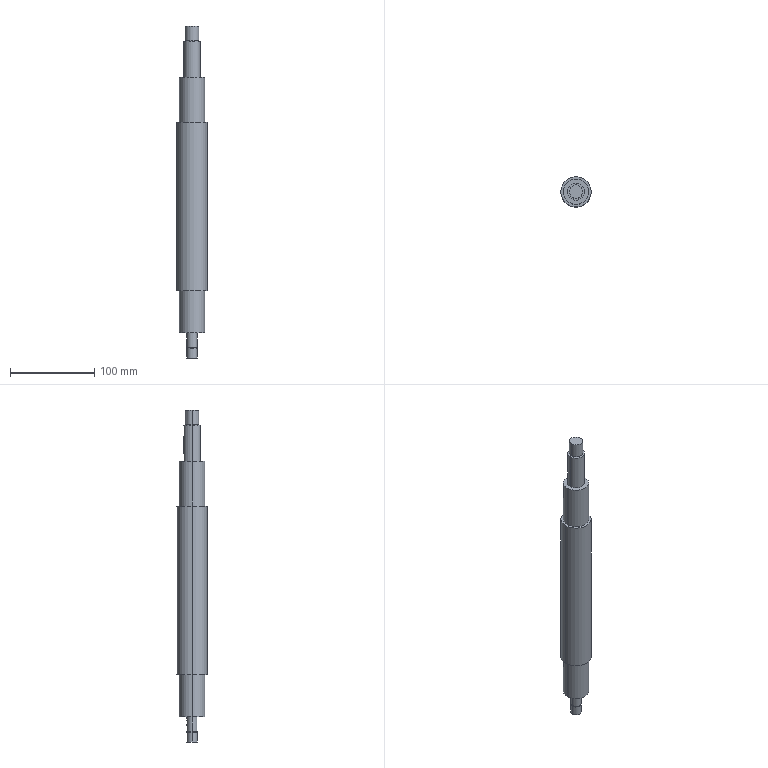Part | SolidWorks | features ICE 9, Extrusion 1 | 1 solid | 40 faces | box 36 x 36 x 394 mm | volume 296771 mm3 | cylinder 24 | plane 16 | commonest cylinder face diameters 2 x6 12 x4 30 x4 10 x2 14 x2 16 x2
STEP:
#1=CARTESIAN_POINT('',(8.,0.,364.));
#2=VERTEX_POINT('',#1);
#3=CARTESIAN_POINT('',(-8.,0.,364.));
#4=VERTEX_POINT('',#3);
#5=CARTESIAN_POINT('',(0.,0.,364.));
#6=DIRECTION('',(0.,0.,1.));
#7=DIRECTION('',(1.,0.,0.));
#8=AXIS2_PLACEMENT_3D('',#5,#6,#7);
#9=CIRCLE('',#8,8.);
#10=EDGE_CURVE('',#2,#4,#9,.T.);
#11=ORIENTED_EDGE('',*,*,#10,.F.);
#12=CARTESIAN_POINT('',(8.,0.,347.));
#13=VERTEX_POINT('',#12);
#14=CARTESIAN_POINT('',(8.,0.,364.));
#15=DIRECTION('',(0.,0.,-1.));
#16=VECTOR('',#15,1000.);
#17=LINE('',#14,#16);
#18=EDGE_CURVE('',#2,#13,#17,.T.);
#19=ORIENTED_EDGE('',*,*,#18,.T.);
#20=CARTESIAN_POINT('',(-8.,0.,347.));
#21=VERTEX_POINT('',#20);
#22=CARTESIAN_POINT('',(0.,0.,347.));
#23=DIRECTION('',(0.,0.,1.));
#24=DIRECTION('',(1.,0.,0.));
#25=AXIS2_PLACEMENT_3D('',#22,#23,#24);
#26=CIRCLE('',#25,8.);
#27=EDGE_CURVE('',#13,#21,#26,.T.);
#28=ORIENTED_EDGE('',*,*,#27,.T.);
#29=CARTESIAN_POINT('',(-8.,0.,364.));
#30=DIRECTION('',(0.,0.,-1.));
#31=VECTOR('',#30,1000.);
#32=LINE('',#29,#31);
#33=EDGE_CURVE('',#4,#21,#32,.T.);
#34=ORIENTED_EDGE('',*,*,#33,.F.);
#35=EDGE_LOOP('',(#11,#19,#28,#34));
#36=FACE_OUTER_BOUND('',#35,.T.);
#37=CARTESIAN_POINT('',(0.,0.,364.));
#38=DIRECTION('',(0.,0.,-1.));
#39=DIRECTION('',(-1.,0.,0.));
#40=AXIS2_PLACEMENT_3D('',#37,#38,#39);
#41=CYLINDRICAL_SURFACE('',#40,8.);
#42=ADVANCED_FACE('',(#36),#41,.T.);
#43=CARTESIAN_POINT('',(7.,0.,347.));
#44=VERTEX_POINT('',#43);
#45=CARTESIAN_POINT('',(-7.,0.,347.));
#46=VERTEX_POINT('',#45);
#47=CARTESIAN_POINT('',(0.,0.,347.));
#48=DIRECTION('',(0.,0.,1.));
#49=DIRECTION('',(1.,0.,0.));
#50=AXIS2_PLACEMENT_3D('',#47,#48,#49);
#51=CIRCLE('',#50,7.);
#52=EDGE_CURVE('',#44,#46,#51,.T.);
#53=ORIENTED_EDGE('',*,*,#52,.F.);
#54=CARTESIAN_POINT('',(7.,0.,346.));
#55=VERTEX_POINT('',#54);
#56=CARTESIAN_POINT('',(7.,0.,347.));
#57=DIRECTION('',(0.,0.,-1.));
#58=VECTOR('',#57,1000.);
#59=LINE('',#56,#58);
#60=EDGE_CURVE('',#44,#55,#59,.T.);
#61=ORIENTED_EDGE('',*,*,#60,.T.);
#62=CARTESIAN_POINT('',(-7.,0.,346.));
#63=VERTEX_POINT('',#62);
#64=CARTESIAN_POINT('',(0.,0.,346.));
#65=DIRECTION('',(0.,0.,1.));
#66=DIRECTION('',(1.,0.,0.));
#67=AXIS2_PLACEMENT_3D('',#64,#65,#66);
#68=CIRCLE('',#67,7.);
#69=EDGE_CURVE('',#55,#63,#68,.T.);
#70=ORIENTED_EDGE('',*,*,#69,.T.);
#71=CARTESIAN_POINT('',(-7.,0.,347.));
#72=DIRECTION('',(0.,0.,-1.));
#73=VECTOR('',#72,1000.);
#74=LINE('',#71,#73);
#75=EDGE_CURVE('',#46,#63,#74,.T.);
#76=ORIENTED_EDGE('',*,*,#75,.F.);
#77=EDGE_LOOP('',(#53,#61,#70,#76));
#78=FACE_OUTER_BOUND('',#77,.T.);
#79=CARTESIAN_POINT('',(0.,0.,347.));
#80=DIRECTION('',(0.,0.,-1.));
#81=DIRECTION('',(-1.,0.,0.));
#82=AXIS2_PLACEMENT_3D('',#79,#80,#81);
#83=CYLINDRICAL_SURFACE('',#82,7.);
#84=ADVANCED_FACE('',(#78),#83,.T.);
#85=CARTESIAN_POINT('',(1.,9.95,313.));
#86=VERTEX_POINT('',#85);
#87=CARTESIAN_POINT('',(0.,10.,312.));
#88=VERTEX_POINT('',#87);
#89=CARTESIAN_POINT('',(1.,9.95,313.));
#90=CARTESIAN_POINT('',(1.,9.95,312.868));
#91=CARTESIAN_POINT('',(0.9739,9.953,312.738));
#92=CARTESIAN_POINT('',(0.8734,9.962,312.496));
#93=CARTESIAN_POINT('',(0.7991,9.968,312.385));
#94=CARTESIAN_POINT('',(0.6146,9.982,312.2));
#95=CARTESIAN_POINT('',(0.503,9.988,312.126));
#96=CARTESIAN_POINT('',(0.2623,9.997,312.026));
#97=CARTESIAN_POINT('',(0.1306,10.,312.));
#98=CARTESIAN_POINT('',(0.,10.,312.));
#99=B_SPLINE_CURVE_WITH_KNOTS('',3,(#89,#90,#91,#92,#93,#94,#95,#96,#97,#98),.UNSPECIFIED.,.F.,.F.,(4,2,2,2,4),(0.,0.0003911,0.0007823,0.001173,0.001565),.UNSPECIFIED.);
#100=EDGE_CURVE('',#86,#88,#99,.T.);
#101=ORIENTED_EDGE('',*,*,#100,.T.);
#102=CARTESIAN_POINT('',(0.,9.,312.));
#103=VERTEX_POINT('',#102);
#104=CARTESIAN_POINT('',(0.,21.,312.));
#105=DIRECTION('',(0.,-1.,0.));
#106=VECTOR('',#105,1000.);
#107=LINE('',#104,#106);
#108=EDGE_CURVE('',#88,#103,#107,.T.);
#109=ORIENTED_EDGE('',*,*,#108,.T.);
#110=CARTESIAN_POINT('',(1.,9.,313.));
#111=VERTEX_POINT('',#110);
#112=CARTESIAN_POINT('',(0.,9.,313.));
#113=DIRECTION('',(0.,1.,0.));
#114=DIRECTION('',(0.,0.,1.));
#115=AXIS2_PLACEMENT_3D('',#112,#113,#114);
#116=CIRCLE('',#115,1.);
#117=EDGE_CURVE('',#111,#103,#116,.T.);
#118=ORIENTED_EDGE('',*,*,#117,.F.);
#119=CARTESIAN_POINT('',(1.,21.,313.));
#120=DIRECTION('',(0.,-1.,0.));
#121=VECTOR('',#120,1000.);
#122=LINE('',#119,#121);
#123=EDGE_CURVE('',#86,#111,#122,.T.);
#124=ORIENTED_EDGE('',*,*,#123,.F.);
#125=EDGE_LOOP('',(#101,#109,#118,#124));
#126=FACE_OUTER_BOUND('',#125,.T.);
#127=CARTESIAN_POINT('',(0.,21.,313.));
#128=DIRECTION('',(0.,-1.,0.));
#129=DIRECTION('',(0.,0.,-1.));
#130=AXIS2_PLACEMENT_3D('',#127,#128,#129);
#131=CYLINDRICAL_SURFACE('',#130,1.);
#132=ADVANCED_FACE('',(#126),#131,.F.);
#133=CARTESIAN_POINT('',(-6.,0.,-30.));
#134=VERTEX_POINT('',#133);
#135=CARTESIAN_POINT('',(6.,0.,-30.));
#136=VERTEX_POINT('',#135);
#137=CARTESIAN_POINT('',(0.,0.,-30.));
#138=DIRECTION('',(0.,0.,-1.));
#139=DIRECTION('',(-1.,0.,0.));
#140=AXIS2_PLACEMENT_3D('',#137,#138,#139);
#141=CIRCLE('',#140,6.);
#142=EDGE_CURVE('',#134,#136,#141,.T.);
#143=ORIENTED_EDGE('',*,*,#142,.F.);
#144=CARTESIAN_POINT('',(-6.,0.,-18.5));
#145=VERTEX_POINT('',#144);
#146=CARTESIAN_POINT('',(-6.,0.,-30.));
#147=DIRECTION('',(0.,0.,1.));
#148=VECTOR('',#147,1000.);
#149=LINE('',#146,#148);
#150=EDGE_CURVE('',#134,#145,#149,.T.);
#151=ORIENTED_EDGE('',*,*,#150,.T.);
#152=CARTESIAN_POINT('',(6.,0.,-18.5));
#153=VERTEX_POINT('',#152);
#154=CARTESIAN_POINT('',(0.,0.,-18.5));
#155=DIRECTION('',(0.,0.,-1.));
#156=DIRECTION('',(-1.,0.,0.));
#157=AXIS2_PLACEMENT_3D('',#154,#155,#156);
#158=CIRCLE('',#157,6.);
#159=EDGE_CURVE('',#145,#153,#158,.T.);
#160=ORIENTED_EDGE('',*,*,#159,.T.);
#161=CARTESIAN_POINT('',(6.,0.,-30.));
#162=DIRECTION('',(0.,0.,1.));
#163=VECTOR('',#162,1000.);
#164=LINE('',#161,#163);
#165=EDGE_CURVE('',#136,#153,#164,.T.);
#166=ORIENTED_EDGE('',*,*,#165,.F.);
#167=EDGE_LOOP('',(#143,#151,#160,#166));
#168=FACE_OUTER_BOUND('',#167,.T.);
#169=CARTESIAN_POINT('',(0.,0.,-30.));
#170=DIRECTION('',(0.,0.,1.));
#171=DIRECTION('',(1.,0.,0.));
#172=AXIS2_PLACEMENT_3D('',#169,#170,#171);
#173=CYLINDRICAL_SURFACE('',#172,6.);
#174=ADVANCED_FACE('',(#168),#173,.T.);
#175=CARTESIAN_POINT('',(-5.,0.,-17.5));
#176=VERTEX_POINT('',#175);
#177=CARTESIAN_POINT('',(5.,0.,-17.5));
#178=VERTEX_POINT('',#177);
#179=CARTESIAN_POINT('',(0.,0.,-17.5));
#180=DIRECTION('',(0.,0.,-1.));
#181=DIRECTION('',(-1.,0.,0.));
#182=AXIS2_PLACEMENT_3D('',#179,#180,#181);
#183=CIRCLE('',#182,5.);
#184=EDGE_CURVE('',#176,#178,#183,.T.);
#185=ORIENTED_EDGE('',*,*,#184,.T.);
#186=CARTESIAN_POINT('',(5.,0.,-18.5));
#187=VERTEX_POINT('',#186);
#188=CARTESIAN_POINT('',(5.,0.,-17.5));
#189=DIRECTION('',(0.,0.,-1.));
#190=VECTOR('',#189,1000.);
#191=LINE('',#188,#190);
#192=EDGE_CURVE('',#178,#187,#191,.T.);
#193=ORIENTED_EDGE('',*,*,#192,.T.);
#194=CARTESIAN_POINT('',(-5.,0.,-18.5));
#195=VERTEX_POINT('',#194);
#196=CARTESIAN_POINT('',(0.,0.,-18.5));
#197=DIRECTION('',(0.,0.,-1.));
#198=DIRECTION('',(-1.,0.,0.));
#199=AXIS2_PLACEMENT_3D('',#196,#197,#198);
#200=CIRCLE('',#199,5.);
#201=EDGE_CURVE('',#195,#187,#200,.T.);
#202=ORIENTED_EDGE('',*,*,#201,.F.);
#203=CARTESIAN_POINT('',(-5.,0.,-17.5));
#204=DIRECTION('',(0.,0.,-1.));
#205=VECTOR('',#204,1000.);
#206=LINE('',#203,#205);
#207=EDGE_CURVE('',#176,#195,#206,.T.);
#208=ORIENTED_EDGE('',*,*,#207,.F.);
#209=EDGE_LOOP('',(#185,#193,#202,#208));
#210=FACE_OUTER_BOUND('',#209,.T.);
#211=CARTESIAN_POINT('',(0.,0.,-17.5));
#212=DIRECTION('',(0.,0.,-1.));
#213=DIRECTION('',(-1.,0.,0.));
#214=AXIS2_PLACEMENT_3D('',#211,#212,#213);
#215=CYLINDRICAL_SURFACE('',#214,5.);
#216=ADVANCED_FACE('',(#210),#215,.T.);
#217=CARTESIAN_POINT('',(1.,5.916,-9.));
#218=VERTEX_POINT('',#217);
#219=CARTESIAN_POINT('',(0.,6.,-10.));
#220=VERTEX_POINT('',#219);
#221=CARTESIAN_POINT('',(1.,5.916,-9.));
#222=CARTESIAN_POINT('',(1.,5.916,-9.132));
#223=CARTESIAN_POINT('',(0.9738,5.921,-9.262));
#224=CARTESIAN_POINT('',(0.8733,5.936,-9.505));
#225=CARTESIAN_POINT('',(0.799,5.947,-9.615));
#226=CARTESIAN_POINT('',(0.6147,5.969,-9.799));
#227=CARTESIAN_POINT('',(0.5032,5.98,-9.874));
#228=CARTESIAN_POINT('',(0.2625,5.995,-9.974));
#229=CARTESIAN_POINT('',(0.1307,6.,-10.));
#230=CARTESIAN_POINT('',(0.,6.,-10.));
#231=B_SPLINE_CURVE_WITH_KNOTS('',3,(#221,#222,#223,#224,#225,#226,#227,#228,#229,#230),.UNSPECIFIED.,.F.,.F.,(4,2,2,2,4),(0.,0.0003916,0.0007832,0.001175,0.001566),.UNSPECIFIED.);
#232=EDGE_CURVE('',#218,#220,#231,.T.);
#233=ORIENTED_EDGE('',*,*,#232,.T.);
#234=CARTESIAN_POINT('',(0.,5.,-10.));
#235=VERTEX_POINT('',#234);
#236=CARTESIAN_POINT('',(0.,15.,-10.));
#237=DIRECTION('',(0.,-1.,0.));
#238=VECTOR('',#237,1000.);
#239=LINE('',#236,#238);
#240=EDGE_CURVE('',#220,#235,#239,.T.);
#241=ORIENTED_EDGE('',*,*,#240,.T.);
#242=CARTESIAN_POINT('',(1.,5.,-9.));
#243=VERTEX_POINT('',#242);
#244=CARTESIAN_POINT('',(0.,5.,-9.));
#245=DIRECTION('',(0.,1.,0.));
#246=DIRECTION('',(0.,0.,1.));
#247=AXIS2_PLACEMENT_3D('',#244,#245,#246);
#248=CIRCLE('',#247,1.);
#249=EDGE_CURVE('',#243,#235,#248,.T.);
#250=ORIENTED_EDGE('',*,*,#249,.F.);
#251=CARTESIAN_POINT('',(1.,15.,-9.));
#252=DIRECTION('',(0.,-1.,0.));
#253=VECTOR('',#252,1000.);
#254=LINE('',#251,#253);
#255=EDGE_CURVE('',#218,#243,#254,.T.);
#256=ORIENTED_EDGE('',*,*,#255,.F.);
#257=EDGE_LOOP('',(#233,#241,#250,#256));
#258=FACE_OUTER_BOUND('',#257,.T.);
#259=CARTESIAN_POINT('',(0.,15.,-9.));
#260=DIRECTION('',(0.,-1.,0.));
#261=DIRECTION('',(0.,0.,-1.));
#262=AXIS2_PLACEMENT_3D('',#259,#260,#261);
#263=CYLINDRICAL_SURFACE('',#262,1.);
#264=ADVANCED_FACE('',(#258),#263,.F.);
#265=CARTESIAN_POINT('',(15.,0.,303.));
#266=VERTEX_POINT('',#265);
#267=CARTESIAN_POINT('',(-15.,0.,303.));
#268=VERTEX_POINT('',#267);
#269=CARTESIAN_POINT('',(0.,0.,303.));
#270=DIRECTION('',(0.,0.,1.));
#271=DIRECTION('',(1.,0.,0.));
#272=AXIS2_PLACEMENT_3D('',#269,#270,#271);
#273=CIRCLE('',#272,15.);
#274=EDGE_CURVE('',#266,#268,#273,.T.);
#275=ORIENTED_EDGE('',*,*,#274,.F.);
#276=CARTESIAN_POINT('',(15.,0.,250.));
#277=VERTEX_POINT('',#276);
#278=CARTESIAN_POINT('',(15.,0.,303.));
#279=DIRECTION('',(0.,0.,-1.));
#280=VECTOR('',#279,1000.);
#281=LINE('',#278,#280);
#282=EDGE_CURVE('',#266,#277,#281,.T.);
#283=ORIENTED_EDGE('',*,*,#282,.T.);
#284=CARTESIAN_POINT('',(-15.,0.,250.));
#285=VERTEX_POINT('',#284);
#286=CARTESIAN_POINT('',(0.,0.,250.));
#287=DIRECTION('',(0.,0.,1.));
#288=DIRECTION('',(1.,0.,0.));
#289=AXIS2_PLACEMENT_3D('',#286,#287,#288);
#290=CIRCLE('',#289,15.);
#291=EDGE_CURVE('',#277,#285,#290,.T.);
#292=ORIENTED_EDGE('',*,*,#291,.T.);
#293=CARTESIAN_POINT('',(-15.,0.,303.));
#294=DIRECTION('',(0.,0.,-1.));
#295=VECTOR('',#294,1000.);
#296=LINE('',#293,#295);
#297=EDGE_CURVE('',#268,#285,#296,.T.);
#298=ORIENTED_EDGE('',*,*,#297,.F.);
#299=EDGE_LOOP('',(#275,#283,#292,#298));
#300=FACE_OUTER_BOUND('',#299,.T.);
#301=CARTESIAN_POINT('',(0.,0.,303.));
#302=DIRECTION('',(0.,0.,-1.));
#303=DIRECTION('',(-1.,0.,0.));
#304=AXIS2_PLACEMENT_3D('',#301,#302,#303);
#305=CYLINDRICAL_SURFACE('',#304,15.);
#306=ADVANCED_FACE('',(#300),#305,.T.);
#307=CARTESIAN_POINT('',(18.,0.,250.));
#308=VERTEX_POINT('',#307);
#309=CARTESIAN_POINT('',(-18.,0.,250.));
#310=VERTEX_POINT('',#309);
#311=CARTESIAN_POINT('',(0.,0.,250.));
#312=DIRECTION('',(0.,0.,1.));
#313=DIRECTION('',(1.,0.,0.));
#314=AXIS2_PLACEMENT_3D('',#311,#312,#313);
#315=CIRCLE('',#314,18.);
#316=EDGE_CURVE('',#308,#310,#315,.T.);
#317=ORIENTED_EDGE('',*,*,#316,.F.);
#318=CARTESIAN_POINT('',(18.,0.,50.));
#319=VERTEX_POINT('',#318);
#320=CARTESIAN_POINT('',(18.,0.,250.));
#321=DIRECTION('',(0.,0.,-1.));
#322=VECTOR('',#321,1000.);
#323=LINE('',#320,#322);
#324=EDGE_CURVE('',#308,#319,#323,.T.);
#325=ORIENTED_EDGE('',*,*,#324,.T.);
#326=CARTESIAN_POINT('',(-18.,0.,50.));
#327=VERTEX_POINT('',#326);
#328=CARTESIAN_POINT('',(0.,0.,50.));
#329=DIRECTION('',(0.,0.,1.));
#330=DIRECTION('',(1.,0.,0.));
#331=AXIS2_PLACEMENT_3D('',#328,#329,#330);
#332=CIRCLE('',#331,18.);
#333=EDGE_CURVE('',#319,#327,#332,.T.);
#334=ORIENTED_EDGE('',*,*,#333,.T.);
#335=CARTESIAN_POINT('',(-18.,0.,250.));
#336=DIRECTION('',(0.,0.,-1.));
#337=VECTOR('',#336,1000.);
#338=LINE('',#335,#337);
#339=EDGE_CURVE('',#310,#327,#338,.T.);
#340=ORIENTED_EDGE('',*,*,#339,.F.);
#341=EDGE_LOOP('',(#317,#325,#334,#340));
#342=FACE_OUTER_BOUND('',#341,.T.);
#343=CARTESIAN_POINT('',(0.,0.,250.));
#344=DIRECTION('',(0.,0.,-1.));
#345=DIRECTION('',(-1.,0.,0.));
#346=AXIS2_PLACEMENT_3D('',#343,#344,#345);
#347=CYLINDRICAL_SURFACE('',#346,18.);
#348=ADVANCED_FACE('',(#342),#347,.T.);
#349=CARTESIAN_POINT('',(15.,0.,50.));
#350=VERTEX_POINT('',#349);
#351=CARTESIAN_POINT('',(-15.,0.,50.));
#352=VERTEX_POINT('',#351);
#353=CARTESIAN_POINT('',(0.,0.,50.));
#354=DIRECTION('',(0.,0.,1.));
#355=DIRECTION('',(1.,0.,0.));
#356=AXIS2_PLACEMENT_3D('',#353,#354,#355);
#357=CIRCLE('',#356,15.);
#358=EDGE_CURVE('',#350,#352,#357,.T.);
#359=ORIENTED_EDGE('',*,*,#358,.F.);
#360=CARTESIAN_POINT('',(15.,0.,0.));
#361=VERTEX_POINT('',#360);
#362=CARTESIAN_POINT('',(15.,0.,50.));
#363=DIRECTION('',(0.,0.,-1.));
#364=VECTOR('',#363,1000.);
#365=LINE('',#362,#364);
#366=EDGE_CURVE('',#350,#361,#365,.T.);
#367=ORIENTED_EDGE('',*,*,#366,.T.);
#368=CARTESIAN_POINT('',(-15.,0.,0.));
#369=VERTEX_POINT('',#368);
#370=CARTESIAN_POINT('',(0.,0.,0.));
#371=DIRECTION('',(0.,0.,1.));
#372=DIRECTION('',(1.,0.,0.));
#373=AXIS2_PLACEMENT_3D('',#370,#371,#372);
#374=CIRCLE('',#373,15.);
#375=EDGE_CURVE('',#361,#369,#374,.T.);
#376=ORIENTED_EDGE('',*,*,#375,.T.);
#377=CARTESIAN_POINT('',(-15.,0.,50.));
#378=DIRECTION('',(0.,0.,-1.));
#379=VECTOR('',#378,1000.);
#380=LINE('',#377,#379);
#381=EDGE_CURVE('',#352,#369,#380,.T.);
#382=ORIENTED_EDGE('',*,*,#381,.F.);
#383=EDGE_LOOP('',(#359,#367,#376,#382));
#384=FACE_OUTER_BOUND('',#383,.T.);
#385=CARTESIAN_POINT('',(0.,0.,50.));
#386=DIRECTION('',(0.,0.,-1.));
#387=DIRECTION('',(-1.,0.,0.));
#388=AXIS2_PLACEMENT_3D('',#385,#386,#387);
#389=CYLINDRICAL_SURFACE('',#388,15.);
#390=ADVANCED_FACE('',(#384),#389,.T.);
#391=ORIENTED_EDGE('',*,*,#232,.F.);
#392=CARTESIAN_POINT('',(1.,5.916,-5.));
#393=VERTEX_POINT('',#392);
#394=CARTESIAN_POINT('',(1.,5.916,-30.));
#395=DIRECTION('',(0.,0.,1.));
#396=VECTOR('',#395,1000.);
#397=LINE('',#394,#396);
#398=EDGE_CURVE('',#218,#393,#397,.T.);
#399=ORIENTED_EDGE('',*,*,#398,.T.);
#400=CARTESIAN_POINT('',(-1.,5.916,-5.));
#401=VERTEX_POINT('',#400);
#402=CARTESIAN_POINT('',(-1.,5.916,-5.));
#403=CARTESIAN_POINT('',(-1.,5.916,-4.868));
#404=CARTESIAN_POINT('',(-0.9739,5.921,-4.738));
#405=CARTESIAN_POINT('',(-0.8734,5.936,-4.496));
#406=CARTESIAN_POINT('',(-0.7992,5.947,-4.385));
#407=CARTESIAN_POINT('',(-0.615,5.969,-4.201));
#408=CARTESIAN_POINT('',(-0.5037,5.98,-4.126));
#409=CARTESIAN_POINT('',(-0.2632,5.995,-4.027));
#410=CARTESIAN_POINT('',(-0.1314,6.,-4.));
#411=CARTESIAN_POINT('',(0.1299,6.,-4.));
#412=CARTESIAN_POINT('',(0.2611,5.996,-4.026));
#413=CARTESIAN_POINT('',(0.5035,5.98,-4.126));
#414=CARTESIAN_POINT('',(0.6135,5.969,-4.199));
#415=CARTESIAN_POINT('',(0.7999,5.947,-4.386));
#416=CARTESIAN_POINT('',(0.8733,5.936,-4.496));
#417=CARTESIAN_POINT('',(0.9737,5.921,-4.737));
#418=CARTESIAN_POINT('',(1.,5.916,-4.868));
#419=CARTESIAN_POINT('',(1.,5.916,-5.));
#420=B_SPLINE_CURVE_WITH_KNOTS('',3,(#402,#403,#404,#405,#406,#407,#408,#409,#410,#411,#412,#413,#414,#415,#416,#417,#418,#419),.UNSPECIFIED.,.F.,.F.,(4,2,2,2,2,2,2,2,4),(0.,0.0003914,0.0007828,0.001174,0.001566,0.001957,0.002348,0.00274,0.003131),.UNSPECIFIED.);
#421=EDGE_CURVE('',#401,#393,#420,.T.);
#422=ORIENTED_EDGE('',*,*,#421,.F.);
#423=CARTESIAN_POINT('',(-1.,5.916,-9.));
#424=VERTEX_POINT('',#423);
#425=CARTESIAN_POINT('',(-1.,5.916,-30.));
#426=DIRECTION('',(0.,0.,1.));
#427=VECTOR('',#426,1000.);
#428=LINE('',#425,#427);
#429=EDGE_CURVE('',#424,#401,#428,.T.);
#430=ORIENTED_EDGE('',*,*,#429,.F.);
#431=CARTESIAN_POINT('',(0.,6.,-10.));
#432=CARTESIAN_POINT('',(-0.1306,6.,-10.));
#433=CARTESIAN_POINT('',(-0.2617,5.996,-9.974));
#434=CARTESIAN_POINT('',(-0.5039,5.98,-9.874));
#435=CARTESIAN_POINT('',(-0.6139,5.969,-9.8));
#436=CARTESIAN_POINT('',(-0.8,5.947,-9.614));
#437=CARTESIAN_POINT('',(-0.8734,5.936,-9.504));
#438=CARTESIAN_POINT('',(-0.9738,5.921,-9.263));
#439=CARTESIAN_POINT('',(-1.,5.916,-9.132));
#440=CARTESIAN_POINT('',(-1.,5.916,-9.));
#441=B_SPLINE_CURVE_WITH_KNOTS('',3,(#431,#432,#433,#434,#435,#436,#437,#438,#439,#440),.UNSPECIFIED.,.F.,.F.,(4,2,2,2,4),(0.001566,0.001958,0.002349,0.00274,0.003131),.UNSPECIFIED.);
#442=EDGE_CURVE('',#220,#424,#441,.T.);
#443=ORIENTED_EDGE('',*,*,#442,.F.);
#444=EDGE_LOOP('',(#391,#399,#422,#430,#443));
#445=FACE_BOUND('',#444,.T.);
#446=CARTESIAN_POINT('',(-6.,0.,-17.5));
#447=VERTEX_POINT('',#446);
#448=CARTESIAN_POINT('',(6.,0.,-17.5));
#449=VERTEX_POINT('',#448);
#450=CARTESIAN_POINT('',(0.,0.,-17.5));
#451=DIRECTION('',(0.,0.,-1.));
#452=DIRECTION('',(-1.,0.,0.));
#453=AXIS2_PLACEMENT_3D('',#450,#451,#452);
#454=CIRCLE('',#453,6.);
#455=EDGE_CURVE('',#447,#449,#454,.T.);
#456=ORIENTED_EDGE('',*,*,#455,.F.);
#457=CARTESIAN_POINT('',(-6.,0.,0.));
#458=VERTEX_POINT('',#457);
#459=CARTESIAN_POINT('',(-6.,0.,-30.));
#460=DIRECTION('',(0.,0.,1.));
#461=VECTOR('',#460,1000.);
#462=LINE('',#459,#461);
#463=EDGE_CURVE('',#447,#458,#462,.T.);
#464=ORIENTED_EDGE('',*,*,#463,.T.);
#465=CARTESIAN_POINT('',(6.,0.,0.));
#466=VERTEX_POINT('',#465);
#467=CARTESIAN_POINT('',(0.,0.,0.));
#468=DIRECTION('',(0.,0.,-1.));
#469=DIRECTION('',(1.,0.,0.));
#470=AXIS2_PLACEMENT_3D('',#467,#468,#469);
#471=CIRCLE('',#470,6.);
#472=EDGE_CURVE('',#458,#466,#471,.T.);
#473=ORIENTED_EDGE('',*,*,#472,.T.);
#474=CARTESIAN_POINT('',(6.,0.,-30.));
#475=DIRECTION('',(0.,0.,1.));
#476=VECTOR('',#475,1000.);
#477=LINE('',#474,#476);
#478=EDGE_CURVE('',#449,#466,#477,.T.);
#479=ORIENTED_EDGE('',*,*,#478,.F.);
#480=EDGE_LOOP('',(#456,#464,#473,#479));
#481=FACE_OUTER_BOUND('',#480,.T.);
#482=CARTESIAN_POINT('',(0.,0.,-30.));
#483=DIRECTION('',(0.,0.,1.));
#484=DIRECTION('',(1.,0.,0.));
#485=AXIS2_PLACEMENT_3D('',#482,#483,#484);
#486=CYLINDRICAL_SURFACE('',#485,6.);
#487=ADVANCED_FACE('',(#445,#481),#486,.T.);
#488=CARTESIAN_POINT('',(-1.,9.95,313.));
#489=VERTEX_POINT('',#488);
#490=CARTESIAN_POINT('',(-1.,9.95,331.));
#491=VERTEX_POINT('',#490);
#492=CARTESIAN_POINT('',(-1.,9.95,346.));
#493=DIRECTION('',(0.,0.,1.));
#494=VECTOR('',#493,1000.);
#495=LINE('',#492,#494);
#496=EDGE_CURVE('',#489,#491,#495,.T.);
#497=ORIENTED_EDGE('',*,*,#496,.F.);
#498=CARTESIAN_POINT('',(0.,10.,312.));
#499=CARTESIAN_POINT('',(-0.1305,10.,312.));
#500=CARTESIAN_POINT('',(-0.2615,9.997,312.026));
#501=CARTESIAN_POINT('',(-0.5036,9.988,312.126));
#502=CARTESIAN_POINT('',(-0.6135,9.982,312.199));
#503=CARTESIAN_POINT('',(-0.8002,9.968,312.386));
#504=CARTESIAN_POINT('',(-0.8735,9.962,312.496));
#505=CARTESIAN_POINT('',(-0.9739,9.953,312.738));
#506=CARTESIAN_POINT('',(-1.,9.95,312.868));
#507=CARTESIAN_POINT('',(-1.,9.95,313.));
#508=B_SPLINE_CURVE_WITH_KNOTS('',3,(#498,#499,#500,#501,#502,#503,#504,#505,#506,#507),.UNSPECIFIED.,.F.,.F.,(4,2,2,2,4),(0.001565,0.001955,0.002346,0.002737,0.003128),.UNSPECIFIED.);
#509=EDGE_CURVE('',#88,#489,#508,.T.);
#510=ORIENTED_EDGE('',*,*,#509,.F.);
#511=ORIENTED_EDGE('',*,*,#100,.F.);
#512=CARTESIAN_POINT('',(1.,9.95,331.));
#513=VERTEX_POINT('',#512);
#514=CARTESIAN_POINT('',(1.,9.95,346.));
#515=DIRECTION('',(0.,0.,1.));
#516=VECTOR('',#515,1000.);
#517=LINE('',#514,#516);
#518=EDGE_CURVE('',#86,#513,#517,.T.);
#519=ORIENTED_EDGE('',*,*,#518,.T.);
#520=CARTESIAN_POINT('',(-1.,9.95,331.));
#521=CARTESIAN_POINT('',(-1.,9.95,331.132));
#522=CARTESIAN_POINT('',(-0.9739,9.953,331.262));
#523=CARTESIAN_POINT('',(-0.8736,9.962,331.504));
#524=CARTESIAN_POINT('',(-0.7993,9.968,331.615));
#525=CARTESIAN_POINT('',(-0.6149,9.982,331.799));
#526=CARTESIAN_POINT('',(-0.5034,9.988,331.874));
#527=CARTESIAN_POINT('',(-0.2628,9.997,331.974));
#528=CARTESIAN_POINT('',(-0.1312,10.,332.));
#529=CARTESIAN_POINT('',(0.1298,10.,332.));
#530=CARTESIAN_POINT('',(0.2609,9.997,331.974));
#531=CARTESIAN_POINT('',(0.5031,9.988,331.874));
#532=CARTESIAN_POINT('',(0.6132,9.982,331.801));
#533=CARTESIAN_POINT('',(0.8,9.968,331.614));
#534=CARTESIAN_POINT('',(0.8734,9.962,331.504));
#535=CARTESIAN_POINT('',(0.9739,9.953,331.262));
#536=CARTESIAN_POINT('',(1.,9.95,331.132));
#537=CARTESIAN_POINT('',(1.,9.95,331.));
#538=B_SPLINE_CURVE_WITH_KNOTS('',3,(#520,#521,#522,#523,#524,#525,#526,#527,#528,#529,#530,#531,#532,#533,#534,#535,#536,#537),.UNSPECIFIED.,.F.,.F.,(4,2,2,2,2,2,2,2,4),(0.,0.000391,0.0007819,0.001173,0.001564,0.001955,0.002346,0.002737,0.003128),.UNSPECIFIED.);
#539=EDGE_CURVE('',#491,#513,#538,.T.);
#540=ORIENTED_EDGE('',*,*,#539,.F.);
#541=EDGE_LOOP('',(#497,#510,#511,#519,#540));
#542=FACE_BOUND('',#541,.T.);
#543=CARTESIAN_POINT('',(10.,0.,346.));
#544=VERTEX_POINT('',#543);
#545=CARTESIAN_POINT('',(-10.,0.,346.));
#546=VERTEX_POINT('',#545);
#547=CARTESIAN_POINT('',(0.,0.,346.));
#548=DIRECTION('',(0.,0.,1.));
#549=DIRECTION('',(1.,0.,0.));
#550=AXIS2_PLACEMENT_3D('',#547,#548,#549);
#551=CIRCLE('',#550,10.);
#552=EDGE_CURVE('',#544,#546,#551,.T.);
#553=ORIENTED_EDGE('',*,*,#552,.F.);
#554=CARTESIAN_POINT('',(10.,0.,303.));
#555=VERTEX_POINT('',#554);
#556=CARTESIAN_POINT('',(10.,0.,346.));
#557=DIRECTION('',(0.,0.,-1.));
#558=VECTOR('',#557,1000.);
#559=LINE('',#556,#558);
#560=EDGE_CURVE('',#544,#555,#559,.T.);
#561=ORIENTED_EDGE('',*,*,#560,.T.);
#562=CARTESIAN_POINT('',(-10.,0.,303.));
#563=VERTEX_POINT('',#562);
#564=CARTESIAN_POINT('',(0.,0.,303.));
#565=DIRECTION('',(0.,0.,1.));
#566=DIRECTION('',(1.,0.,0.));
#567=AXIS2_PLACEMENT_3D('',#564,#565,#566);
#568=CIRCLE('',#567,10.);
#569=EDGE_CURVE('',#555,#563,#568,.T.);
#570=ORIENTED_EDGE('',*,*,#569,.T.);
#571=CARTESIAN_POINT('',(-10.,0.,346.));
#572=DIRECTION('',(0.,0.,-1.));
#573=VECTOR('',#572,1000.);
#574=LINE('',#571,#573);
#575=EDGE_CURVE('',#546,#563,#574,.T.);
#576=ORIENTED_EDGE('',*,*,#575,.F.);
#577=EDGE_LOOP('',(#553,#561,#570,#576));
#578=FACE_OUTER_BOUND('',#577,.T.);
#579=CARTESIAN_POINT('',(0.,0.,346.));
#580=DIRECTION('',(0.,0.,-1.));
#581=DIRECTION('',(-1.,0.,0.));
#582=AXIS2_PLACEMENT_3D('',#579,#580,#581);
#583=CYLINDRICAL_SURFACE('',#582,10.);
#584=ADVANCED_FACE('',(#542,#578),#583,.T.);
#585=ORIENTED_EDGE('',*,*,#560,.F.);
#586=CARTESIAN_POINT('',(0.,0.,346.));
#587=DIRECTION('',(0.,0.,1.));
#588=DIRECTION('',(1.,0.,0.));
#589=AXIS2_PLACEMENT_3D('',#586,#587,#588);
#590=CIRCLE('',#589,10.);
#591=EDGE_CURVE('',#546,#544,#590,.T.);
#592=ORIENTED_EDGE('',*,*,#591,.F.);
#593=ORIENTED_EDGE('',*,*,#575,.T.);
#594=CARTESIAN_POINT('',(0.,0.,303.));
#595=DIRECTION('',(0.,0.,1.));
#596=DIRECTION('',(1.,0.,0.));
#597=AXIS2_PLACEMENT_3D('',#594,#595,#596);
#598=CIRCLE('',#597,10.);
#599=EDGE_CURVE('',#563,#555,#598,.T.);
#600=ORIENTED_EDGE('',*,*,#599,.T.);
#601=EDGE_LOOP('',(#585,#592,#593,#600));
#602=FACE_OUTER_BOUND('',#601,.T.);
#603=CARTESIAN_POINT('',(0.,0.,346.));
#604=DIRECTION('',(0.,0.,-1.));
#605=DIRECTION('',(-1.,0.,0.));
#606=AXIS2_PLACEMENT_3D('',#603,#604,#605);
#607=CYLINDRICAL_SURFACE('',#606,10.);
#608=ADVANCED_FACE('',(#602),#607,.T.);
#609=ORIENTED_EDGE('',*,*,#463,.F.);
#610=CARTESIAN_POINT('',(0.,0.,-17.5));
#611=DIRECTION('',(0.,0.,-1.));
#612=DIRECTION('',(-1.,0.,0.));
#613=AXIS2_PLACEMENT_3D('',#610,#611,#612);
#614=CIRCLE('',#613,6.);
#615=EDGE_CURVE('',#449,#447,#614,.T.);
#616=ORIENTED_EDGE('',*,*,#615,.F.);
#617=ORIENTED_EDGE('',*,*,#478,.T.);
#618=CARTESIAN_POINT('',(0.,0.,0.));
#619=DIRECTION('',(0.,0.,-1.));
#620=DIRECTION('',(1.,0.,0.));
#621=AXIS2_PLACEMENT_3D('',#618,#619,#620);
#622=CIRCLE('',#621,6.);
#623=EDGE_CURVE('',#466,#458,#622,.T.);
#624=ORIENTED_EDGE('',*,*,#623,.T.);
#625=EDGE_LOOP('',(#609,#616,#617,#624));
#626=FACE_OUTER_BOUND('',#625,.T.);
#627=CARTESIAN_POINT('',(0.,0.,-30.));
#628=DIRECTION('',(0.,0.,1.));
#629=DIRECTION('',(1.,0.,0.));
#630=AXIS2_PLACEMENT_3D('',#627,#628,#629);
#631=CYLINDRICAL_SURFACE('',#630,6.);
#632=ADVANCED_FACE('',(#626),#631,.T.);
#633=ORIENTED_EDGE('',*,*,#366,.F.);
#634=CARTESIAN_POINT('',(0.,0.,50.));
#635=DIRECTION('',(0.,0.,1.));
#636=DIRECTION('',(1.,0.,0.));
#637=AXIS2_PLACEMENT_3D('',#634,#635,#636);
#638=CIRCLE('',#637,15.);
#639=EDGE_CURVE('',#352,#350,#638,.T.);
#640=ORIENTED_EDGE('',*,*,#639,.F.);
#641=ORIENTED_EDGE('',*,*,#381,.T.);
#642=CARTESIAN_POINT('',(0.,0.,0.));
#643=DIRECTION('',(0.,0.,1.));
#644=DIRECTION('',(1.,0.,0.));
#645=AXIS2_PLACEMENT_3D('',#642,#643,#644);
#646=CIRCLE('',#645,15.);
#647=EDGE_CURVE('',#369,#361,#646,.T.);
#648=ORIENTED_EDGE('',*,*,#647,.T.);
#649=EDGE_LOOP('',(#633,#640,#641,#648));
#650=FACE_OUTER_BOUND('',#649,.T.);
#651=CARTESIAN_POINT('',(0.,0.,50.));
#652=DIRECTION('',(0.,0.,-1.));
#653=DIRECTION('',(-1.,0.,0.));
#654=AXIS2_PLACEMENT_3D('',#651,#652,#653);
#655=CYLINDRICAL_SURFACE('',#654,15.);
#656=ADVANCED_FACE('',(#650),#655,.T.);
#657=ORIENTED_EDGE('',*,*,#623,.F.);
#658=ORIENTED_EDGE('',*,*,#472,.F.);
#659=EDGE_LOOP('',(#657,#658));
#660=FACE_BOUND('',#659,.T.);
#661=ORIENTED_EDGE('',*,*,#647,.F.);
#662=ORIENTED_EDGE('',*,*,#375,.F.);
#663=EDGE_LOOP('',(#661,#662));
#664=FACE_OUTER_BOUND('',#663,.T.);
#665=CARTESIAN_POINT('',(0.,0.,0.));
#666=DIRECTION('',(0.,0.,1.));
#667=DIRECTION('',(1.,0.,0.));
#668=AXIS2_PLACEMENT_3D('',#665,#666,#667);
#669=PLANE('',#668);
#670=ADVANCED_FACE('',(#660,#664),#669,.F.);
#671=ORIENTED_EDGE('',*,*,#324,.F.);
#672=CARTESIAN_POINT('',(0.,0.,250.));
#673=DIRECTION('',(0.,0.,1.));
#674=DIRECTION('',(1.,0.,0.));
#675=AXIS2_PLACEMENT_3D('',#672,#673,#674);
#676=CIRCLE('',#675,18.);
#677=EDGE_CURVE('',#310,#308,#676,.T.);
#678=ORIENTED_EDGE('',*,*,#677,.F.);
#679=ORIENTED_EDGE('',*,*,#339,.T.);
#680=CARTESIAN_POINT('',(0.,0.,50.));
#681=DIRECTION('',(0.,0.,1.));
#682=DIRECTION('',(1.,0.,0.));
#683=AXIS2_PLACEMENT_3D('',#680,#681,#682);
#684=CIRCLE('',#683,18.);
#685=EDGE_CURVE('',#327,#319,#684,.T.);
#686=ORIENTED_EDGE('',*,*,#685,.T.);
#687=EDGE_LOOP('',(#671,#678,#679,#686));
#688=FACE_OUTER_BOUND('',#687,.T.);
#689=CARTESIAN_POINT('',(0.,0.,250.));
#690=DIRECTION('',(0.,0.,-1.));
#691=DIRECTION('',(-1.,0.,0.));
#692=AXIS2_PLACEMENT_3D('',#689,#690,#691);
#693=CYLINDRICAL_SURFACE('',#692,18.);
#694=ADVANCED_FACE('',(#688),#693,.T.);
#695=CARTESIAN_POINT('',(0.,0.,250.));
#696=DIRECTION('',(0.,0.,1.));
#697=DIRECTION('',(1.,0.,0.));
#698=AXIS2_PLACEMENT_3D('',#695,#696,#697);
#699=CIRCLE('',#698,15.);
#700=EDGE_CURVE('',#285,#277,#699,.T.);
#701=ORIENTED_EDGE('',*,*,#700,.F.);
#702=ORIENTED_EDGE('',*,*,#291,.F.);
#703=EDGE_LOOP('',(#701,#702));
#704=FACE_BOUND('',#703,.T.);
#705=ORIENTED_EDGE('',*,*,#677,.T.);
#706=ORIENTED_EDGE('',*,*,#316,.T.);
#707=EDGE_LOOP('',(#705,#706));
#708=FACE_OUTER_BOUND('',#707,.T.);
#709=CARTESIAN_POINT('',(0.,0.,250.));
#710=DIRECTION('',(0.,0.,1.));
#711=DIRECTION('',(1.,0.,0.));
#712=AXIS2_PLACEMENT_3D('',#709,#710,#711);
#713=PLANE('',#712);
#714=ADVANCED_FACE('',(#704,#708),#713,.T.);
#715=ORIENTED_EDGE('',*,*,#639,.T.);
#716=ORIENTED_EDGE('',*,*,#358,.T.);
#717=EDGE_LOOP('',(#715,#716));
#718=FACE_BOUND('',#717,.T.);
#719=ORIENTED_EDGE('',*,*,#685,.F.);
#720=ORIENTED_EDGE('',*,*,#333,.F.);
#721=EDGE_LOOP('',(#719,#720));
#722=FACE_OUTER_BOUND('',#721,.T.);
#723=CARTESIAN_POINT('',(0.,0.,50.));
#724=DIRECTION('',(0.,0.,1.));
#725=DIRECTION('',(1.,0.,0.));
#726=AXIS2_PLACEMENT_3D('',#723,#724,#725);
#727=PLANE('',#726);
#728=ADVANCED_FACE('',(#718,#722),#727,.F.);
#729=ORIENTED_EDGE('',*,*,#282,.F.);
#730=CARTESIAN_POINT('',(0.,0.,303.));
#731=DIRECTION('',(0.,0.,1.));
#732=DIRECTION('',(1.,0.,0.));
#733=AXIS2_PLACEMENT_3D('',#730,#731,#732);
#734=CIRCLE('',#733,15.);
#735=EDGE_CURVE('',#268,#266,#734,.T.);
#736=ORIENTED_EDGE('',*,*,#735,.F.);
#737=ORIENTED_EDGE('',*,*,#297,.T.);
#738=ORIENTED_EDGE('',*,*,#700,.T.);
#739=EDGE_LOOP('',(#729,#736,#737,#738));
#740=FACE_OUTER_BOUND('',#739,.T.);
#741=CARTESIAN_POINT('',(0.,0.,303.));
#742=DIRECTION('',(0.,0.,-1.));
#743=DIRECTION('',(-1.,0.,0.));
#744=AXIS2_PLACEMENT_3D('',#741,#742,#743);
#745=CYLINDRICAL_SURFACE('',#744,15.);
#746=ADVANCED_FACE('',(#740),#745,.T.);
#747=ORIENTED_EDGE('',*,*,#599,.F.);
#748=ORIENTED_EDGE('',*,*,#569,.F.);
#749=EDGE_LOOP('',(#747,#748));
#750=FACE_BOUND('',#749,.T.);
#751=ORIENTED_EDGE('',*,*,#735,.T.);
#752=ORIENTED_EDGE('',*,*,#274,.T.);
#753=EDGE_LOOP('',(#751,#752));
#754=FACE_OUTER_BOUND('',#753,.T.);
#755=CARTESIAN_POINT('',(0.,0.,303.));
#756=DIRECTION('',(0.,0.,1.));
#757=DIRECTION('',(1.,0.,0.));
#758=AXIS2_PLACEMENT_3D('',#755,#756,#757);
#759=PLANE('',#758);
#760=ADVANCED_FACE('',(#750,#754),#759,.T.);
#761=ORIENTED_EDGE('',*,*,#240,.F.);
#762=ORIENTED_EDGE('',*,*,#442,.T.);
#763=CARTESIAN_POINT('',(-1.,5.,-9.));
#764=VERTEX_POINT('',#763);
#765=CARTESIAN_POINT('',(-1.,15.,-9.));
#766=DIRECTION('',(0.,-1.,0.));
#767=VECTOR('',#766,1000.);
#768=LINE('',#765,#767);
#769=EDGE_CURVE('',#424,#764,#768,.T.);
#770=ORIENTED_EDGE('',*,*,#769,.T.);
#771=CARTESIAN_POINT('',(0.,5.,-9.));
#772=DIRECTION('',(0.,1.,0.));
#773=DIRECTION('',(0.,0.,1.));
#774=AXIS2_PLACEMENT_3D('',#771,#772,#773);
#775=CIRCLE('',#774,1.);
#776=EDGE_CURVE('',#235,#764,#775,.T.);
#777=ORIENTED_EDGE('',*,*,#776,.F.);
#778=EDGE_LOOP('',(#761,#762,#770,#777));
#779=FACE_OUTER_BOUND('',#778,.T.);
#780=CARTESIAN_POINT('',(0.,15.,-9.));
#781=DIRECTION('',(0.,-1.,0.));
#782=DIRECTION('',(0.,0.,-1.));
#783=AXIS2_PLACEMENT_3D('',#780,#781,#782);
#784=CYLINDRICAL_SURFACE('',#783,1.);
#785=ADVANCED_FACE('',(#779),#784,.F.);
#786=ORIENTED_EDGE('',*,*,#429,.T.);
#787=CARTESIAN_POINT('',(-1.,5.,-5.));
#788=VERTEX_POINT('',#787);
#789=CARTESIAN_POINT('',(-1.,15.,-5.));
#790=DIRECTION('',(0.,-1.,0.));
#791=VECTOR('',#790,1000.);
#792=LINE('',#789,#791);
#793=EDGE_CURVE('',#401,#788,#792,.T.);
#794=ORIENTED_EDGE('',*,*,#793,.T.);
#795=CARTESIAN_POINT('',(-1.,5.,0.));
#796=DIRECTION('',(0.,0.,1.));
#797=VECTOR('',#796,1000.);
#798=LINE('',#795,#797);
#799=EDGE_CURVE('',#764,#788,#798,.T.);
#800=ORIENTED_EDGE('',*,*,#799,.F.);
#801=ORIENTED_EDGE('',*,*,#769,.F.);
#802=EDGE_LOOP('',(#786,#794,#800,#801));
#803=FACE_OUTER_BOUND('',#802,.T.);
#804=CARTESIAN_POINT('',(-1.,15.,0.));
#805=DIRECTION('',(1.,0.,0.));
#806=DIRECTION('',(0.,0.,-1.));
#807=AXIS2_PLACEMENT_3D('',#804,#805,#806);
#808=PLANE('',#807);
#809=ADVANCED_FACE('',(#803),#808,.T.);
#810=ORIENTED_EDGE('',*,*,#421,.T.);
#811=CARTESIAN_POINT('',(1.,5.,-5.));
#812=VERTEX_POINT('',#811);
#813=CARTESIAN_POINT('',(1.,15.,-5.));
#814=DIRECTION('',(0.,-1.,0.));
#815=VECTOR('',#814,1000.);
#816=LINE('',#813,#815);
#817=EDGE_CURVE('',#393,#812,#816,.T.);
#818=ORIENTED_EDGE('',*,*,#817,.T.);
#819=CARTESIAN_POINT('',(0.,5.,-5.));
#820=DIRECTION('',(0.,1.,0.));
#821=DIRECTION('',(0.,0.,1.));
#822=AXIS2_PLACEMENT_3D('',#819,#820,#821);
#823=CIRCLE('',#822,1.);
#824=EDGE_CURVE('',#788,#812,#823,.T.);
#825=ORIENTED_EDGE('',*,*,#824,.F.);
#826=ORIENTED_EDGE('',*,*,#793,.F.);
#827=EDGE_LOOP('',(#810,#818,#825,#826));
#828=FACE_OUTER_BOUND('',#827,.T.);
#829=CARTESIAN_POINT('',(0.,15.,-5.));
#830=DIRECTION('',(0.,-1.,0.));
#831=DIRECTION('',(0.,0.,-1.));
#832=AXIS2_PLACEMENT_3D('',#829,#830,#831);
#833=CYLINDRICAL_SURFACE('',#832,1.);
#834=ADVANCED_FACE('',(#828),#833,.F.);
#835=ORIENTED_EDGE('',*,*,#255,.T.);
#836=CARTESIAN_POINT('',(1.,5.,0.));
#837=DIRECTION('',(0.,0.,1.));
#838=VECTOR('',#837,1000.);
#839=LINE('',#836,#838);
#840=EDGE_CURVE('',#243,#812,#839,.T.);
#841=ORIENTED_EDGE('',*,*,#840,.T.);
#842=ORIENTED_EDGE('',*,*,#817,.F.);
#843=ORIENTED_EDGE('',*,*,#398,.F.);
#844=EDGE_LOOP('',(#835,#841,#842,#843));
#845=FACE_OUTER_BOUND('',#844,.T.);
#846=CARTESIAN_POINT('',(1.,15.,0.));
#847=DIRECTION('',(1.,0.,0.));
#848=DIRECTION('',(0.,0.,-1.));
#849=AXIS2_PLACEMENT_3D('',#846,#847,#848);
#850=PLANE('',#849);
#851=ADVANCED_FACE('',(#845),#850,.F.);
#852=ORIENTED_EDGE('',*,*,#249,.T.);
#853=ORIENTED_EDGE('',*,*,#776,.T.);
#854=ORIENTED_EDGE('',*,*,#799,.T.);
#855=ORIENTED_EDGE('',*,*,#824,.T.);
#856=ORIENTED_EDGE('',*,*,#840,.F.);
#857=EDGE_LOOP('',(#852,#853,#854,#855,#856));
#858=FACE_OUTER_BOUND('',#857,.T.);
#859=CARTESIAN_POINT('',(0.,5.,0.));
#860=DIRECTION('',(0.,1.,0.));
#861=DIRECTION('',(0.,0.,1.));
#862=AXIS2_PLACEMENT_3D('',#859,#860,#861);
#863=PLANE('',#862);
#864=ADVANCED_FACE('',(#858),#863,.T.);
#865=ORIENTED_EDGE('',*,*,#184,.F.);
#866=CARTESIAN_POINT('',(0.,0.,-17.5));
#867=DIRECTION('',(0.,0.,-1.));
#868=DIRECTION('',(-1.,0.,0.));
#869=AXIS2_PLACEMENT_3D('',#866,#867,#868);
#870=CIRCLE('',#869,5.);
#871=EDGE_CURVE('',#178,#176,#870,.T.);
#872=ORIENTED_EDGE('',*,*,#871,.F.);
#873=EDGE_LOOP('',(#865,#872));
#874=FACE_BOUND('',#873,.T.);
#875=ORIENTED_EDGE('',*,*,#615,.T.);
#876=ORIENTED_EDGE('',*,*,#455,.T.);
#877=EDGE_LOOP('',(#875,#876));
#878=FACE_OUTER_BOUND('',#877,.T.);
#879=CARTESIAN_POINT('',(0.,0.,-17.5));
#880=DIRECTION('',(0.,0.,-1.));
#881=DIRECTION('',(-1.,0.,0.));
#882=AXIS2_PLACEMENT_3D('',#879,#880,#881);
#883=PLANE('',#882);
#884=ADVANCED_FACE('',(#874,#878),#883,.T.);
#885=ORIENTED_EDGE('',*,*,#201,.T.);
#886=CARTESIAN_POINT('',(0.,0.,-18.5));
#887=DIRECTION('',(0.,0.,-1.));
#888=DIRECTION('',(-1.,0.,0.));
#889=AXIS2_PLACEMENT_3D('',#886,#887,#888);
#890=CIRCLE('',#889,5.);
#891=EDGE_CURVE('',#187,#195,#890,.T.);
#892=ORIENTED_EDGE('',*,*,#891,.T.);
#893=EDGE_LOOP('',(#885,#892));
#894=FACE_BOUND('',#893,.T.);
#895=CARTESIAN_POINT('',(0.,0.,-18.5));
#896=DIRECTION('',(0.,0.,-1.));
#897=DIRECTION('',(-1.,0.,0.));
#898=AXIS2_PLACEMENT_3D('',#895,#896,#897);
#899=CIRCLE('',#898,6.);
#900=EDGE_CURVE('',#153,#145,#899,.T.);
#901=ORIENTED_EDGE('',*,*,#900,.F.);
#902=ORIENTED_EDGE('',*,*,#159,.F.);
#903=EDGE_LOOP('',(#901,#902));
#904=FACE_OUTER_BOUND('',#903,.T.);
#905=CARTESIAN_POINT('',(0.,0.,-18.5));
#906=DIRECTION('',(0.,0.,-1.));
#907=DIRECTION('',(-1.,0.,0.));
#908=AXIS2_PLACEMENT_3D('',#905,#906,#907);
#909=PLANE('',#908);
#910=ADVANCED_FACE('',(#894,#904),#909,.F.);
#911=ORIENTED_EDGE('',*,*,#192,.F.);
#912=ORIENTED_EDGE('',*,*,#871,.T.);
#913=ORIENTED_EDGE('',*,*,#207,.T.);
#914=ORIENTED_EDGE('',*,*,#891,.F.);
#915=EDGE_LOOP('',(#911,#912,#913,#914));
#916=FACE_OUTER_BOUND('',#915,.T.);
#917=CARTESIAN_POINT('',(0.,0.,-17.5));
#918=DIRECTION('',(0.,0.,-1.));
#919=DIRECTION('',(-1.,0.,0.));
#920=AXIS2_PLACEMENT_3D('',#917,#918,#919);
#921=CYLINDRICAL_SURFACE('',#920,5.);
#922=ADVANCED_FACE('',(#916),#921,.T.);
#923=CARTESIAN_POINT('',(0.,0.,-30.));
#924=DIRECTION('',(0.,0.,-1.));
#925=DIRECTION('',(-1.,0.,0.));
#926=AXIS2_PLACEMENT_3D('',#923,#924,#925);
#927=CIRCLE('',#926,6.);
#928=EDGE_CURVE('',#136,#134,#927,.T.);
#929=ORIENTED_EDGE('',*,*,#928,.T.);
#930=ORIENTED_EDGE('',*,*,#142,.T.);
#931=EDGE_LOOP('',(#929,#930));
#932=FACE_OUTER_BOUND('',#931,.T.);
#933=CARTESIAN_POINT('',(0.,0.,-30.));
#934=DIRECTION('',(0.,0.,-1.));
#935=DIRECTION('',(-1.,0.,0.));
#936=AXIS2_PLACEMENT_3D('',#933,#934,#935);
#937=PLANE('',#936);
#938=ADVANCED_FACE('',(#932),#937,.T.);
#939=ORIENTED_EDGE('',*,*,#150,.F.);
#940=ORIENTED_EDGE('',*,*,#928,.F.);
#941=ORIENTED_EDGE('',*,*,#165,.T.);
#942=ORIENTED_EDGE('',*,*,#900,.T.);
#943=EDGE_LOOP('',(#939,#940,#941,#942));
#944=FACE_OUTER_BOUND('',#943,.T.);
#945=CARTESIAN_POINT('',(0.,0.,-30.));
#946=DIRECTION('',(0.,0.,1.));
#947=DIRECTION('',(1.,0.,0.));
#948=AXIS2_PLACEMENT_3D('',#945,#946,#947);
#949=CYLINDRICAL_SURFACE('',#948,6.);
#950=ADVANCED_FACE('',(#944),#949,.T.);
#951=ORIENTED_EDGE('',*,*,#591,.T.);
#952=ORIENTED_EDGE('',*,*,#552,.T.);
#953=EDGE_LOOP('',(#951,#952));
#954=FACE_OUTER_BOUND('',#953,.T.);
#955=CARTESIAN_POINT('',(0.,0.,346.));
#956=DIRECTION('',(0.,0.,1.));
#957=DIRECTION('',(1.,0.,0.));
#958=AXIS2_PLACEMENT_3D('',#955,#956,#957);
#959=CIRCLE('',#958,7.);
#960=EDGE_CURVE('',#63,#55,#959,.T.);
#961=ORIENTED_EDGE('',*,*,#960,.F.);
#962=ORIENTED_EDGE('',*,*,#69,.F.);
#963=EDGE_LOOP('',(#961,#962));
#964=FACE_BOUND('',#963,.T.);
#965=CARTESIAN_POINT('',(0.,0.,346.));
#966=DIRECTION('',(0.,0.,1.));
#967=DIRECTION('',(1.,0.,0.));
#968=AXIS2_PLACEMENT_3D('',#965,#966,#967);
#969=PLANE('',#968);
#970=ADVANCED_FACE('',(#954,#964),#969,.T.);
#971=ORIENTED_EDGE('',*,*,#496,.T.);
#972=CARTESIAN_POINT('',(-1.,9.,331.));
#973=VERTEX_POINT('',#972);
#974=CARTESIAN_POINT('',(-1.,21.,331.));
#975=DIRECTION('',(0.,-1.,0.));
#976=VECTOR('',#975,1000.);
#977=LINE('',#974,#976);
#978=EDGE_CURVE('',#491,#973,#977,.T.);
#979=ORIENTED_EDGE('',*,*,#978,.T.);
#980=CARTESIAN_POINT('',(-1.,9.,313.));
#981=VERTEX_POINT('',#980);
#982=CARTESIAN_POINT('',(-1.,9.,0.));
#983=DIRECTION('',(0.,0.,1.));
#984=VECTOR('',#983,1000.);
#985=LINE('',#982,#984);
#986=EDGE_CURVE('',#981,#973,#985,.T.);
#987=ORIENTED_EDGE('',*,*,#986,.F.);
#988=CARTESIAN_POINT('',(-1.,21.,313.));
#989=DIRECTION('',(0.,-1.,0.));
#990=VECTOR('',#989,1000.);
#991=LINE('',#988,#990);
#992=EDGE_CURVE('',#489,#981,#991,.T.);
#993=ORIENTED_EDGE('',*,*,#992,.F.);
#994=EDGE_LOOP('',(#971,#979,#987,#993));
#995=FACE_OUTER_BOUND('',#994,.T.);
#996=CARTESIAN_POINT('',(-1.,21.,0.));
#997=DIRECTION('',(1.,0.,0.));
#998=DIRECTION('',(0.,0.,-1.));
#999=AXIS2_PLACEMENT_3D('',#996,#997,#998);
#1000=PLANE('',#999);
#1001=ADVANCED_FACE('',(#995),#1000,.T.);
#1002=ORIENTED_EDGE('',*,*,#539,.T.);
#1003=CARTESIAN_POINT('',(1.,9.,331.));
#1004=VERTEX_POINT('',#1003);
#1005=CARTESIAN_POINT('',(1.,21.,331.));
#1006=DIRECTION('',(0.,-1.,0.));
#1007=VECTOR('',#1006,1000.);
#1008=LINE('',#1005,#1007);
#1009=EDGE_CURVE('',#513,#1004,#1008,.T.);
#1010=ORIENTED_EDGE('',*,*,#1009,.T.);
#1011=CARTESIAN_POINT('',(0.,9.,331.));
#1012=DIRECTION('',(0.,1.,0.));
#1013=DIRECTION('',(0.,0.,1.));
#1014=AXIS2_PLACEMENT_3D('',#1011,#1012,#1013);
#1015=CIRCLE('',#1014,1.);
#1016=EDGE_CURVE('',#973,#1004,#1015,.T.);
#1017=ORIENTED_EDGE('',*,*,#1016,.F.);
#1018=ORIENTED_EDGE('',*,*,#978,.F.);
#1019=EDGE_LOOP('',(#1002,#1010,#1017,#1018));
#1020=FACE_OUTER_BOUND('',#1019,.T.);
#1021=CARTESIAN_POINT('',(0.,21.,331.));
#1022=DIRECTION('',(0.,-1.,0.));
#1023=DIRECTION('',(0.,0.,-1.));
#1024=AXIS2_PLACEMENT_3D('',#1021,#1022,#1023);
#1025=CYLINDRICAL_SURFACE('',#1024,1.);
#1026=ADVANCED_FACE('',(#1020),#1025,.F.);
#1027=ORIENTED_EDGE('',*,*,#123,.T.);
#1028=CARTESIAN_POINT('',(1.,9.,0.));
#1029=DIRECTION('',(0.,0.,1.));
#1030=VECTOR('',#1029,1000.);
#1031=LINE('',#1028,#1030);
#1032=EDGE_CURVE('',#111,#1004,#1031,.T.);
#1033=ORIENTED_EDGE('',*,*,#1032,.T.);
#1034=ORIENTED_EDGE('',*,*,#1009,.F.);
#1035=ORIENTED_EDGE('',*,*,#518,.F.);
#1036=EDGE_LOOP('',(#1027,#1033,#1034,#1035));
#1037=FACE_OUTER_BOUND('',#1036,.T.);
#1038=CARTESIAN_POINT('',(1.,21.,0.));
#1039=DIRECTION('',(1.,0.,0.));
#1040=DIRECTION('',(0.,0.,-1.));
#1041=AXIS2_PLACEMENT_3D('',#1038,#1039,#1040);
#1042=PLANE('',#1041);
#1043=ADVANCED_FACE('',(#1037),#1042,.F.);
#1044=ORIENTED_EDGE('',*,*,#108,.F.);
#1045=ORIENTED_EDGE('',*,*,#509,.T.);
#1046=ORIENTED_EDGE('',*,*,#992,.T.);
#1047=CARTESIAN_POINT('',(0.,9.,313.));
#1048=DIRECTION('',(0.,1.,0.));
#1049=DIRECTION('',(0.,0.,1.));
#1050=AXIS2_PLACEMENT_3D('',#1047,#1048,#1049);
#1051=CIRCLE('',#1050,1.);
#1052=EDGE_CURVE('',#103,#981,#1051,.T.);
#1053=ORIENTED_EDGE('',*,*,#1052,.F.);
#1054=EDGE_LOOP('',(#1044,#1045,#1046,#1053));
#1055=FACE_OUTER_BOUND('',#1054,.T.);
#1056=CARTESIAN_POINT('',(0.,21.,313.));
#1057=DIRECTION('',(0.,-1.,0.));
#1058=DIRECTION('',(0.,0.,-1.));
#1059=AXIS2_PLACEMENT_3D('',#1056,#1057,#1058);
#1060=CYLINDRICAL_SURFACE('',#1059,1.);
#1061=ADVANCED_FACE('',(#1055),#1060,.F.);
#1062=ORIENTED_EDGE('',*,*,#986,.T.);
#1063=ORIENTED_EDGE('',*,*,#1016,.T.);
#1064=ORIENTED_EDGE('',*,*,#1032,.F.);
#1065=ORIENTED_EDGE('',*,*,#117,.T.);
#1066=ORIENTED_EDGE('',*,*,#1052,.T.);
#1067=EDGE_LOOP('',(#1062,#1063,#1064,#1065,#1066));
#1068=FACE_OUTER_BOUND('',#1067,.T.);
#1069=CARTESIAN_POINT('',(0.,9.,0.));
#1070=DIRECTION('',(0.,1.,0.));
#1071=DIRECTION('',(0.,0.,1.));
#1072=AXIS2_PLACEMENT_3D('',#1069,#1070,#1071);
#1073=PLANE('',#1072);
#1074=ADVANCED_FACE('',(#1068),#1073,.T.);
#1075=CARTESIAN_POINT('',(0.,0.,347.));
#1076=DIRECTION('',(0.,0.,1.));
#1077=DIRECTION('',(1.,0.,0.));
#1078=AXIS2_PLACEMENT_3D('',#1075,#1076,#1077);
#1079=CIRCLE('',#1078,7.);
#1080=EDGE_CURVE('',#46,#44,#1079,.T.);
#1081=ORIENTED_EDGE('',*,*,#1080,.T.);
#1082=ORIENTED_EDGE('',*,*,#52,.T.);
#1083=EDGE_LOOP('',(#1081,#1082));
#1084=FACE_BOUND('',#1083,.T.);
#1085=CARTESIAN_POINT('',(0.,0.,347.));
#1086=DIRECTION('',(0.,0.,1.));
#1087=DIRECTION('',(1.,0.,0.));
#1088=AXIS2_PLACEMENT_3D('',#1085,#1086,#1087);
#1089=CIRCLE('',#1088,8.);
#1090=EDGE_CURVE('',#21,#13,#1089,.T.);
#1091=ORIENTED_EDGE('',*,*,#1090,.F.);
#1092=ORIENTED_EDGE('',*,*,#27,.F.);
#1093=EDGE_LOOP('',(#1091,#1092));
#1094=FACE_OUTER_BOUND('',#1093,.T.);
#1095=CARTESIAN_POINT('',(0.,0.,347.));
#1096=DIRECTION('',(0.,0.,1.));
#1097=DIRECTION('',(1.,0.,0.));
#1098=AXIS2_PLACEMENT_3D('',#1095,#1096,#1097);
#1099=PLANE('',#1098);
#1100=ADVANCED_FACE('',(#1084,#1094),#1099,.F.);
#1101=ORIENTED_EDGE('',*,*,#60,.F.);
#1102=ORIENTED_EDGE('',*,*,#1080,.F.);
#1103=ORIENTED_EDGE('',*,*,#75,.T.);
#1104=ORIENTED_EDGE('',*,*,#960,.T.);
#1105=EDGE_LOOP('',(#1101,#1102,#1103,#1104));
#1106=FACE_OUTER_BOUND('',#1105,.T.);
#1107=CARTESIAN_POINT('',(0.,0.,347.));
#1108=DIRECTION('',(0.,0.,-1.));
#1109=DIRECTION('',(-1.,0.,0.));
#1110=AXIS2_PLACEMENT_3D('',#1107,#1108,#1109);
#1111=CYLINDRICAL_SURFACE('',#1110,7.);
#1112=ADVANCED_FACE('',(#1106),#1111,.T.);
#1113=CARTESIAN_POINT('',(0.,0.,364.));
#1114=DIRECTION('',(0.,0.,1.));
#1115=DIRECTION('',(1.,0.,0.));
#1116=AXIS2_PLACEMENT_3D('',#1113,#1114,#1115);
#1117=CIRCLE('',#1116,8.);
#1118=EDGE_CURVE('',#4,#2,#1117,.T.);
#1119=ORIENTED_EDGE('',*,*,#1118,.T.);
#1120=ORIENTED_EDGE('',*,*,#10,.T.);
#1121=EDGE_LOOP('',(#1119,#1120));
#1122=FACE_OUTER_BOUND('',#1121,.T.);
#1123=CARTESIAN_POINT('',(0.,0.,364.));
#1124=DIRECTION('',(0.,0.,1.));
#1125=DIRECTION('',(1.,0.,0.));
#1126=AXIS2_PLACEMENT_3D('',#1123,#1124,#1125);
#1127=PLANE('',#1126);
#1128=ADVANCED_FACE('',(#1122),#1127,.T.);
#1129=ORIENTED_EDGE('',*,*,#18,.F.);
#1130=ORIENTED_EDGE('',*,*,#1118,.F.);
#1131=ORIENTED_EDGE('',*,*,#33,.T.);
#1132=ORIENTED_EDGE('',*,*,#1090,.T.);
#1133=EDGE_LOOP('',(#1129,#1130,#1131,#1132));
#1134=FACE_OUTER_BOUND('',#1133,.T.);
#1135=CARTESIAN_POINT('',(0.,0.,364.));
#1136=DIRECTION('',(0.,0.,-1.));
#1137=DIRECTION('',(-1.,0.,0.));
#1138=AXIS2_PLACEMENT_3D('',#1135,#1136,#1137);
#1139=CYLINDRICAL_SURFACE('',#1138,8.);
#1140=ADVANCED_FACE('',(#1134),#1139,.T.);
#1141=CLOSED_SHELL('',(#42,#84,#132,#174,#216,#264,#306,#348,#390,#487,#584,#608,#632,#656,#670,#694,#714,#728,#746,#760,#785,#809,#834,#851,#864,#884,#910,#922,#938,#950,#970,#1001,#1026,#1043,#1061,#1074,#1100,#1112,#1128,#1140));
#1142=MANIFOLD_SOLID_BREP('',#1141);
#1143=CARTESIAN_POINT('',(0.,0.,0.));
#1144=DIRECTION('',(0.,0.,1.));
#1145=DIRECTION('',(1.,0.,0.));
#1146=AXIS2_PLACEMENT_3D('',#1143,#1144,#1145);
#1147=(LENGTH_UNIT()NAMED_UNIT(*)SI_UNIT(.MILLI.,.METRE.));
#1148=UNCERTAINTY_MEASURE_WITH_UNIT(LENGTH_MEASURE(0.00001),#1147,'','');
#1149=(NAMED_UNIT(*)PLANE_ANGLE_UNIT()SI_UNIT($,.RADIAN.));
#1150=(NAMED_UNIT(*)SI_UNIT($,.STERADIAN.)SOLID_ANGLE_UNIT());
#1151=(GEOMETRIC_REPRESENTATION_CONTEXT(3)GLOBAL_UNCERTAINTY_ASSIGNED_CONTEXT((#1148))GLOBAL_UNIT_ASSIGNED_CONTEXT((#1147,#1149,#1150))REPRESENTATION_CONTEXT('',''));
#1152=ADVANCED_BREP_SHAPE_REPRESENTATION('',(#1142,#1146),#1151);